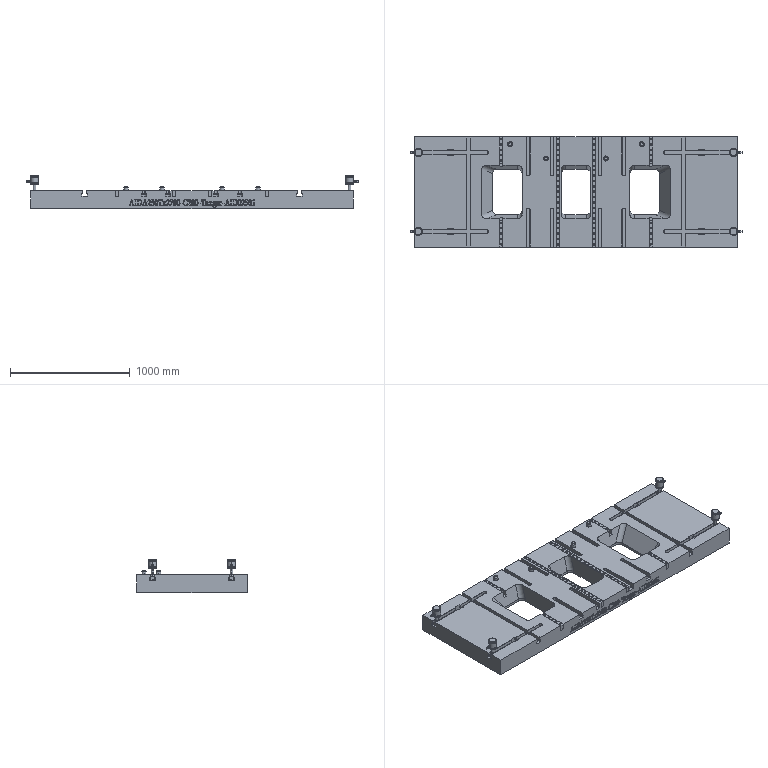Part | CATIA | 15 solids | 3827 faces | volume 311750025 mm3 | spline 1376 | plane 832 | cylinder 781 | other 349 | sphere 248 | cone 188 | torus 53 | commonest cylinder face diameters 66 x424 2 x52 21 x48 5 x44 38 x24 80 x24